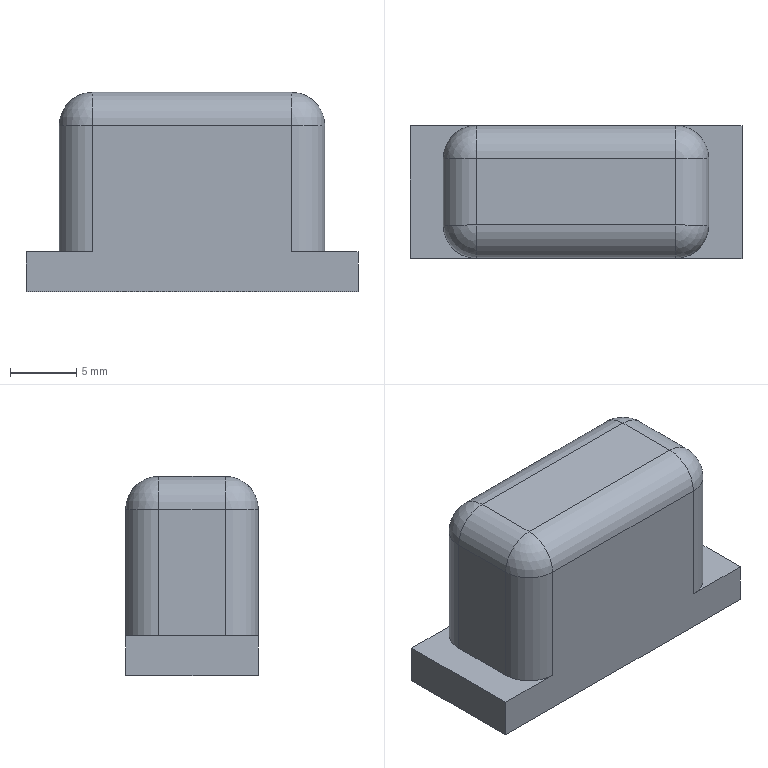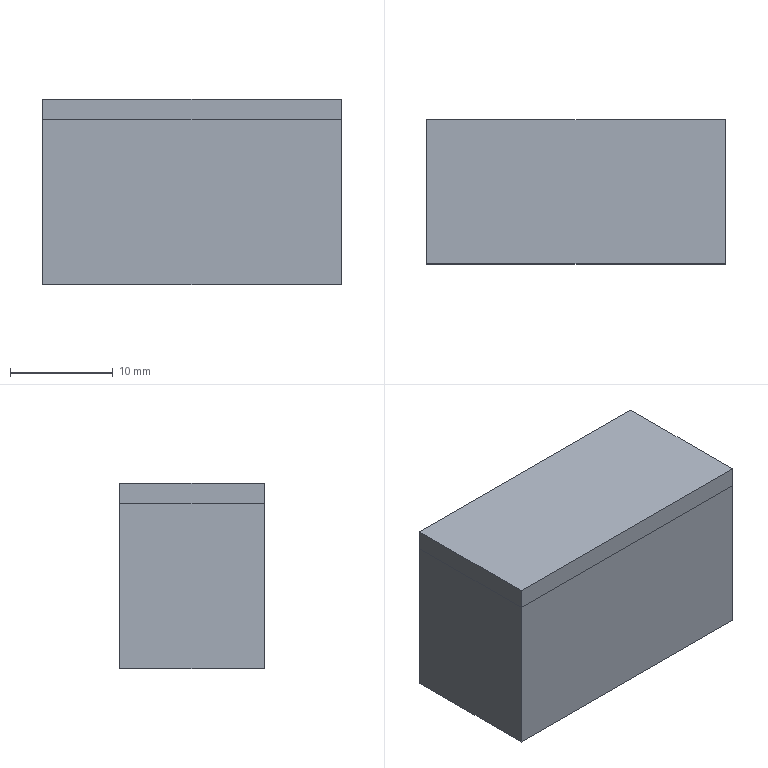CAM job | NX | 3-axis milling | part box 25 x 10 x 15 mm | stock box 29 x 14 x 18 mm
Tools:
number,name,description,diameter,corner_radius,flute_length,length,flutes
1,D50,Milling Tool-5 Parameters,50.0,0.0,50.0,75.0,2
10,D10,Milling Tool-5 Parameters,10.0,0.0,50.0,75.0,2
11,D10JING,Milling Tool-5 Parameters,10.0,0.0,50.0,75.0,2
5,D4R0.5,Milling Tool-5 Parameters,4.0,0.5,50.0,75.0,2
7,D6A45,Milling Tool-5 Parameters,6.0,0.0,50.0,75.0,2
Operations:
program,operation,operation_type,tool,method,geometry_group,spindle_rpm,surface_speed,feed_per_tooth,feed_cut,feed_plunge,cut_length_mm,path_length_mm,cut_time_min,machine_time_min
1,FLOOR_WALL,VolumeBased25DMillingOperation,D50,METHOD,A,4000.0,628.0,0.125,1000.0,100.0,91.0,145.0,0.091,0.0964
1,ZLEVEL_PROFILE,ZLevelMilling,D10,METHOD,A,3500.0,109.0,0.3571,2500.0,1000.0,6362.834,6435.834,2.559,2.566
1,ZLEVEL_PROFILE_COPY,ZLevelMilling,D10JING,METHOD,A,5000.0,157.0,0.12,1200.0,1000.0,108.754,196.754,0.0912,0.1
1,ZLEVEL_PROFILE_COPY_COPY,ZLevelMilling,D10JING,METHOD,A,5000.0,157.0,0.12,1200.0,1000.0,94.516,176.516,0.0794,0.0876
1,ZLEVEL_PROFILE_COPY_1,ZLevelMilling,D4R0.5,METHOD,A,7500.0,94.0,0.2,3000.0,1000.0,2882.016,2943.016,0.9735,0.9796
1,刀补,ZLevelMilling,D10JING,METHOD,A,5000.0,157.0,0.12,1200.0,1000.0,94.716,176.716,0.0795,0.0877
2,FLOOR_WALL_COPY,VolumeBased25DMillingOperation,D50,METHOD,B,4000.0,628.0,0.125,1000.0,100.0,819.0,1961.002,0.819,0.9332
2,PLANAR_MILL,PlanarMilling,D6A45,METHOD,B,8000.0,150.0,0.0781,1250.0,100.0,82.194,141.194,0.0658,0.0717